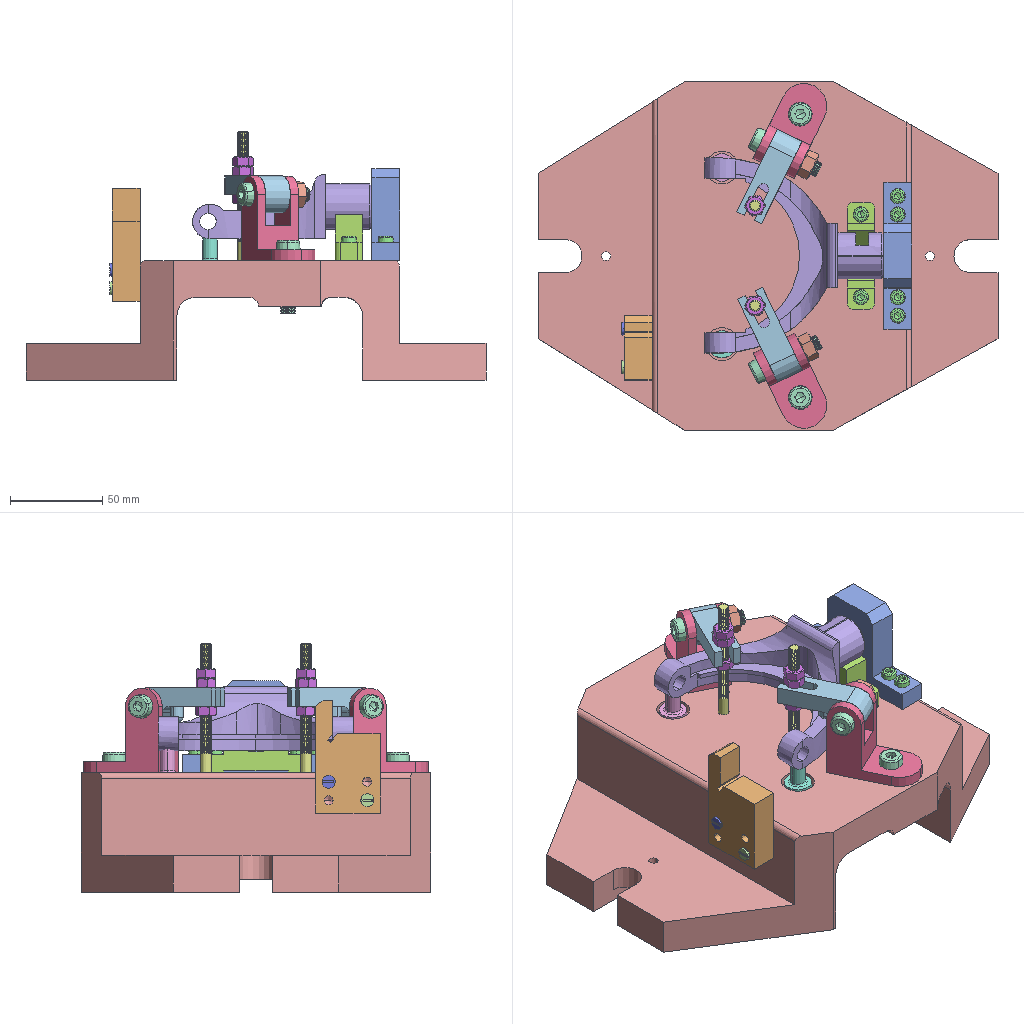Assembly | SolidWorks | 16 different items | 33 placed | box 250 x 190 x 135 mm
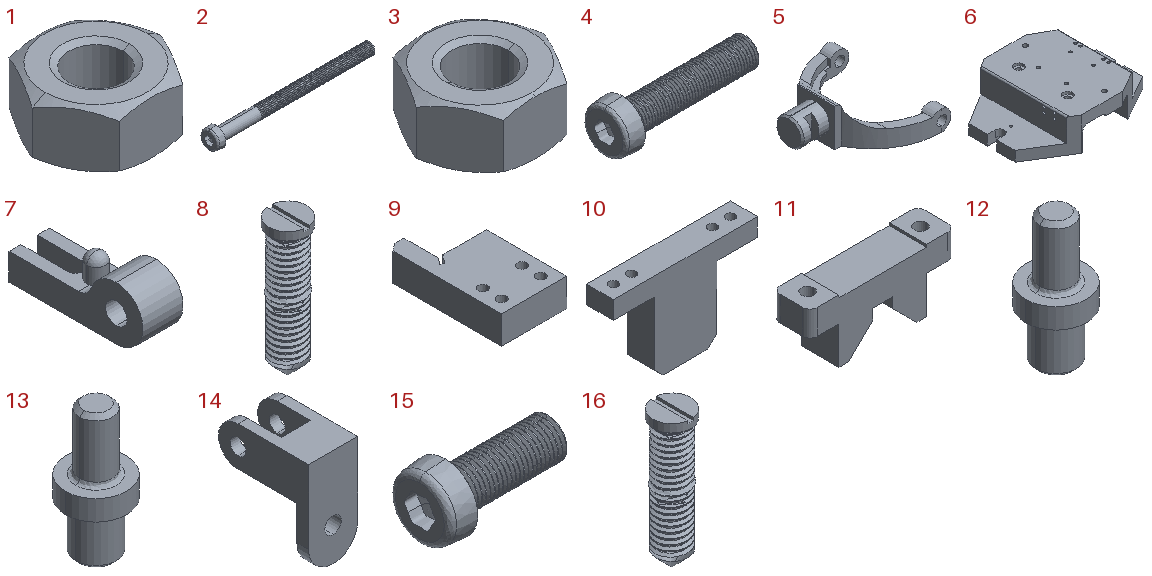Parts list (item | quantity | size | volume | features):
1 | x6 | 11.547 x 10 x 5.2 mm | 340.663 mm3 | features BaseBody 1
2 | x2 | 83.9 x 10 x 10 mm | 2301 mm3 | features BaseBody 1, MoveFace 1
3 | x2 | 15.011 x 13 x 6.8 mm | 739.533 mm3 | features BaseBody 1
4 | x4 | 40 x 13 x 13 mm | 2107 mm3 | features BaseBody 1
5 | x1 | 97.5 x 106 x 35 mm | 48605 mm3 | features BaseBody 1
6 | x1 | 250 x 190 x 65 mm | 1073575 mm3 | features ICE 10, MoveFace 2, BaseBody 1, Cut 1
7 | x2 | 15 x 50 x 20 mm | 7920 mm3 | features ICE 4, Fillet 2, Dome 1, Extrusion 1
8 | x1 | - | - | features RefSurface 1
9 | x1 | 35 x 61.218 x 15 mm | 23648 mm3 | features BaseBody 1
10 | x1 | 80 x 15 x 50 mm | 31840 mm3 | features BaseBody 1
11 | x1 | 58 x 15 x 25 mm | 12562 mm3 | features ICE 2, BaseBody 1, Fillet 1
12 | x1 | 15 x 15 x 32 mm | 2576 mm3 | features BaseBody 1
13 | x1 | 15 x 15 x 32 mm | 2576 mm3 | features BaseBody 1
14 | x2 | 25 x 46 x 50 mm | 17741 mm3 | features ICE 4, Fillet 2, Extrusion 1
15 | x6 | 16.583 x 8.333 x 8.333 mm | 372.356 mm3 | features BaseBody 1, Scale 1
16 | x1 | - | - | features RefSurface 1
Mates (type | each side: item.copy, entity, surface, feature):
Concentric | 11.1 face cylinder Input1 | 15.1 edge
Coincident | 11.1 face plane Input1 | 15.1 face plane Input1
Concentric | 11.1 face cylinder Input1 | 15.2 edge
Coincident | 11.1 face plane Input1 | 15.2 face plane Input1
Concentric | 10.1 face cylinder Input1 | 15.3 edge
Coincident | 10.1 face plane Input1 | 15.3 face plane Input1
Concentric | 10.1 face cylinder Input1 | 15.4 edge
Coincident | 10.1 face plane Input1 | 15.4 face plane Input1
Concentric | 10.1 face cylinder Input1 | 15.5 edge
Coincident | 10.1 face plane Input1 | 15.5 face plane Input1
Concentric | 10.1 face cylinder Input1 | 15.6 edge
Coincident | 10.1 face plane Input1 | 15.6 face plane Input1
Coincident | 6.1 face plane Input1 | 14.1 face plane Boss-Extrude1
Concentric | 6.1 face cylinder Input1 | 14.1 face cylinder Cut-Extrude3
Concentric | 14.1 face cylinder Cut-Extrude2 | 7.1 face cylinder Cut-Extrude1
Coincident | 14.1 face plane Cut-Extrude1 | 7.1 face plane Boss-Extrude1
Parallel | 5.1 face plane Input1 | 7.1 face plane Boss-Extrude1
Concentric | 6.1 face cylinder Cut-Extrude3 | 2.1 face cylinder Input1
Coincident | 6.1 face plane Cut-Extrude5 | 2.1 face plane Input1
Concentric | 1.1 face cylinder Input1 | 1.2 face cylinder Input1
Coincident | 1.1 face plane Input1 | 1.2 face plane Input1
Concentric | 2.1 face cylinder Input1 | 1.1 face cylinder Input1
Coincident | 7.1 face plane Boss-Extrude1 | 1.2 face plane Input1
Concentric | 2.1 face cylinder Input1 | 1.3 edge
Coincident | 7.1 face plane Cut-Extrude2 | 1.3 face plane Input1
Concentric | 14.1 face cylinder Cut-Extrude2 | 4.1 face cylinder Input1
Coincident | 14.1 face plane Boss-Extrude1 | 4.1 face plane Input1
Concentric | 14.1 face cylinder Cut-Extrude3 | 4.2 face cylinder Input1
Coincident | 14.1 face plane Boss-Extrude1 | 4.2 face plane Input1
Concentric | 14.1 face cylinder Fillet3 | 3.1 face cylinder Input1
Coincident | 14.1 face plane Boss-Extrude1 | 3.1 face plane Input1
Concentric | 6.1 face cylinder Input1 | 14.2 face cylinder Cut-Extrude3
Coincident | 6.1 face plane Input1 | 14.2 face plane Boss-Extrude1
Concentric | 14.2 face cylinder Cut-Extrude2 | 7.2 face cylinder Cut-Extrude1
Coincident | 14.2 face plane Cut-Extrude1 | 7.2 face plane Boss-Extrude1
Parallel | 6.1 face plane Input1 | 7.2 face plane Boss-Extrude1
Concentric | 6.1 face cylinder Cut-Extrude4 | 2.2 face cylinder Input1
Coincident | 2.1 face plane Input1 | 2.2 face plane Input1
Concentric | 1.4 face cylinder Input1 | 1.5 face cylinder Input1
Concentric | 1.4 face cylinder Input1 | 1.6 face cylinder Input1
Coincident | 1.4 face plane Input1 | 1.5 face plane Input1
Concentric | 2.2 face cylinder Input1 | 1.4 face cylinder Input1
Coincident | 7.2 face plane Boss-Extrude1 | 1.5 face plane Input1
Coincident | 7.2 face plane Cut-Extrude2 | 1.6 face plane Input1
Concentric | 14.2 face cylinder Cut-Extrude3 | 4.3 face cone Input1
Coincident | 14.2 face plane Boss-Extrude1 | 4.3 face plane Input1
Concentric | 14.2 face cylinder Cut-Extrude2 | 4.4 face cone Input1
Coincident | 14.2 face plane Boss-Extrude1 | 4.4 face plane Input1
Concentric | 14.2 face cylinder Fillet3 | 3.2 face cylinder Input1
Coincident | 14.2 face plane Boss-Extrude1 | 3.2 face plane Input1